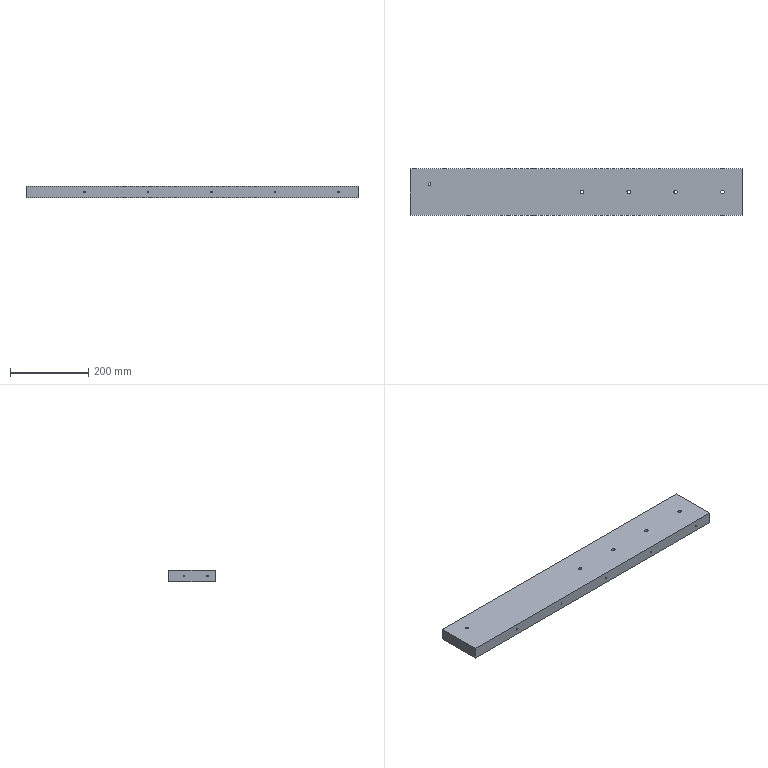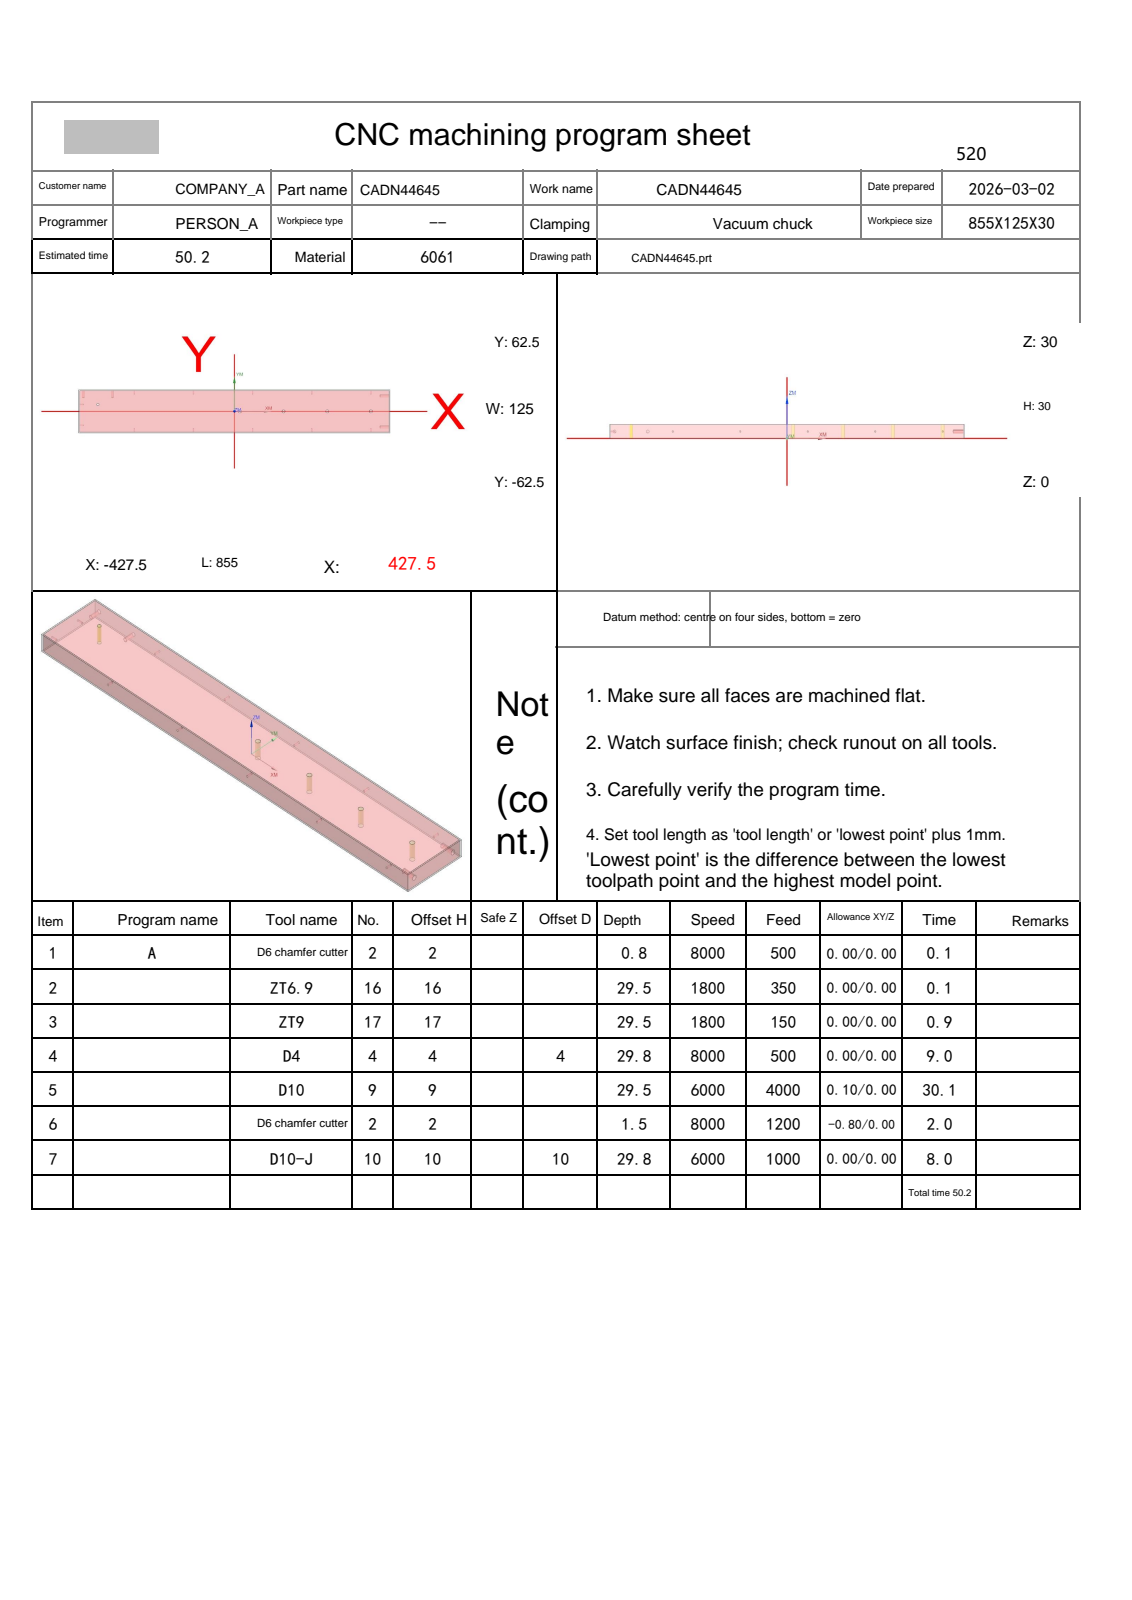NC program | NX | posted by the shop | part box 850 x 120 x 30 mm
Lines 1478 to 2164 of 2164:
N5 T09 M06
(D10  D=10. R=0. H=09 ce=0.10 di=0.00)
G00 G90 G54 X0.0 Y65.1 M03 S6000
G43 H09 Z80.
M08
Z30.5
G01 X425. Z30.392 F4000.
G02 X430.1 Y60. Z30.39 I0.0 J-5.1
G01 Y-60. Z30.36
G02 X425. Y-65.1 Z30.358 I-5.1 J0.0
G01 X-425. Z30.142
G02 X-430.1 Y-60. Z30.14 I0.0 J5.1
G01 Y60. Z30.11
G02 X-425. Y65.1 Z30.108 I5.1 J0.0
G01 X425. Z29.892
G02 X430.1 Y60. Z29.89 I0.0 J-5.1
G01 Y-60. Z29.86
G02 X425. Y-65.1 Z29.858 I-5.1 J0.0
G01 X-425. Z29.642
G02 X-430.1 Y-60. Z29.64 I0.0 J5.1
G01 Y60. Z29.61
G02 X-425. Y65.1 Z29.608 I5.1 J0.0
G01 X425. Z29.392
G02 X430.1 Y60. Z29.39 I0.0 J-5.1
G01 Y-60. Z29.36
G02 X425. Y-65.1 Z29.358 I-5.1 J0.0
G01 X-425. Z29.142
G02 X-430.1 Y-60. Z29.14 I0.0 J5.1
G01 Y60. Z29.11
G02 X-425. Y65.1 Z29.108 I5.1 J0.0
G01 X425. Z28.892
G02 X430.1 Y60. Z28.89 I0.0 J-5.1
G01 Y-60. Z28.86
G02 X425. Y-65.1 Z28.858 I-5.1 J0.0
G01 X-425. Z28.642
G02 X-430.1 Y-60. Z28.64 I0.0 J5.1
G01 Y60. Z28.61
G02 X-425. Y65.1 Z28.608 I5.1 J0.0
G01 X425. Z28.392
G02 X430.1 Y60. Z28.39 I0.0 J-5.1
G01 Y-60. Z28.36
G02 X425. Y-65.1 Z28.358 I-5.1 J0.0
G01 X-425. Z28.142
G02 X-430.1 Y-60. Z28.14 I0.0 J5.1
G01 Y60. Z28.11
G02 X-425. Y65.1 Z28.108 I5.1 J0.0
G01 X425. Z27.892
G02 X430.1 Y60. Z27.89 I0.0 J-5.1
G01 Y-60. Z27.86
G02 X425. Y-65.1 Z27.858 I-5.1 J0.0
G01 X-425. Z27.642
G02 X-430.1 Y-60. Z27.64 I0.0 J5.1
G01 Y60. Z27.61
G02 X-425. Y65.1 Z27.608 I5.1 J0.0
G01 X425. Z27.392
G02 X430.1 Y60. Z27.39 I0.0 J-5.1
G01 Y-60. Z27.36
G02 X425. Y-65.1 Z27.358 I-5.1 J0.0
G01 X-425. Z27.142
G02 X-430.1 Y-60. Z27.14 I0.0 J5.1
G01 Y60. Z27.11
G02 X-425. Y65.1 Z27.108 I5.1 J0.0
G01 X425. Z26.892
G02 X430.1 Y60. Z26.89 I0.0 J-5.1
G01 Y-60. Z26.86
G02 X425. Y-65.1 Z26.858 I-5.1 J0.0
G01 X-425. Z26.642
G02 X-430.1 Y-60. Z26.64 I0.0 J5.1
G01 Y60. Z26.61
G02 X-425. Y65.1 Z26.608 I5.1 J0.0
G01 X425. Z26.392
G02 X430.1 Y60. Z26.39 I0.0 J-5.1
G01 Y-60. Z26.36
G02 X425. Y-65.1 Z26.358 I-5.1 J0.0
G01 X-425. Z26.142
G02 X-430.1 Y-60. Z26.14 I0.0 J5.1
G01 Y60. Z26.11
G02 X-425. Y65.1 Z26.108 I5.1 J0.0
G01 X425. Z25.892
G02 X430.1 Y60. Z25.89 I0.0 J-5.1
G01 Y-60. Z25.86
G02 X425. Y-65.1 Z25.858 I-5.1 J0.0
G01 X-425. Z25.642
G02 X-430.1 Y-60. Z25.64 I0.0 J5.1
G01 Y60. Z25.61
G02 X-425. Y65.1 Z25.608 I5.1 J0.0
G01 X425. Z25.392
G02 X430.1 Y60. Z25.39 I0.0 J-5.1
G01 Y-60. Z25.36
G02 X425. Y-65.1 Z25.358 I-5.1 J0.0
G01 X-425. Z25.142
G02 X-430.1 Y-60. Z25.14 I0.0 J5.1
G01 Y60. Z25.11
G02 X-425. Y65.1 Z25.108 I5.1 J0.0
G01 X425. Z24.892
G02 X430.1 Y60. Z24.89 I0.0 J-5.1
G01 Y-60. Z24.86
G02 X425. Y-65.1 Z24.858 I-5.1 J0.0
G01 X-425. Z24.642
G02 X-430.1 Y-60. Z24.64 I0.0 J5.1
G01 Y60. Z24.61
G02 X-425. Y65.1 Z24.608 I5.1 J0.0
G01 X425. Z24.392
G02 X430.1 Y60. Z24.39 I0.0 J-5.1
G01 Y-60. Z24.36
G02 X425. Y-65.1 Z24.358 I-5.1 J0.0
G01 X-425. Z24.142
G02 X-430.1 Y-60. Z24.14 I0.0 J5.1
G01 Y60. Z24.11
G02 X-425. Y65.1 Z24.108 I5.1 J0.0
G01 X425. Z23.892
G02 X430.1 Y60. Z23.89 I0.0 J-5.1
G01 Y-60. Z23.86
G02 X425. Y-65.1 Z23.858 I-5.1 J0.0
G01 X-425. Z23.642
G02 X-430.1 Y-60. Z23.64 I0.0 J5.1
G01 Y60. Z23.61
G02 X-425. Y65.1 Z23.608 I5.1 J0.0
G01 X425. Z23.392
G02 X430.1 Y60. Z23.39 I0.0 J-5.1
G01 Y-60. Z23.36
G02 X425. Y-65.1 Z23.358 I-5.1 J0.0
G01 X-425. Z23.142
G02 X-430.1 Y-60. Z23.14 I0.0 J5.1
G01 Y60. Z23.11
G02 X-425. Y65.1 Z23.108 I5.1 J0.0
G01 X425. Z22.892
G02 X430.1 Y60. Z22.89 I0.0 J-5.1
G01 Y-60. Z22.86
G02 X425. Y-65.1 Z22.858 I-5.1 J0.0
G01 X-425. Z22.642
G02 X-430.1 Y-60. Z22.64 I0.0 J5.1
G01 Y60. Z22.61
G02 X-425. Y65.1 Z22.608 I5.1 J0.0
G01 X425. Z22.392
G02 X430.1 Y60. Z22.39 I0.0 J-5.1
G01 Y-60. Z22.36
G02 X425. Y-65.1 Z22.358 I-5.1 J0.0
G01 X-425. Z22.142
G02 X-430.1 Y-60. Z22.14 I0.0 J5.1
G01 Y60. Z22.11
G02 X-425. Y65.1 Z22.108 I5.1 J0.0
G01 X425. Z21.892
G02 X430.1 Y60. Z21.89 I0.0 J-5.1
G01 Y-60. Z21.86
G02 X425. Y-65.1 Z21.858 I-5.1 J0.0
G01 X-425. Z21.642
G02 X-430.1 Y-60. Z21.64 I0.0 J5.1
G01 Y60. Z21.61
G02 X-425. Y65.1 Z21.608 I5.1 J0.0
G01 X425. Z21.392
G02 X430.1 Y60. Z21.39 I0.0 J-5.1
G01 Y-60. Z21.36
G02 X425. Y-65.1 Z21.358 I-5.1 J0.0
G01 X-425. Z21.142
G02 X-430.1 Y-60. Z21.14 I0.0 J5.1
G01 Y60. Z21.11
G02 X-425. Y65.1 Z21.108 I5.1 J0.0
G01 X425. Z20.892
G02 X430.1 Y60. Z20.89 I0.0 J-5.1
G01 Y-60. Z20.86
G02 X425. Y-65.1 Z20.858 I-5.1 J0.0
G01 X-425. Z20.642
G02 X-430.1 Y-60. Z20.64 I0.0 J5.1
G01 Y60. Z20.61
G02 X-425. Y65.1 Z20.608 I5.1 J0.0
G01 X425. Z20.392
G02 X430.1 Y60. Z20.39 I0.0 J-5.1
G01 Y-60. Z20.36
G02 X425. Y-65.1 Z20.358 I-5.1 J0.0
G01 X-425. Z20.142
G02 X-430.1 Y-60. Z20.14 I0.0 J5.1
G01 Y60. Z20.11
G02 X-425. Y65.1 Z20.108 I5.1 J0.0
G01 X425. Z19.892
G02 X430.1 Y60. Z19.89 I0.0 J-5.1
G01 Y-60. Z19.86
G02 X425. Y-65.1 Z19.858 I-5.1 J0.0
G01 X-425. Z19.642
G02 X-430.1 Y-60. Z19.64 I0.0 J5.1
G01 Y60. Z19.61
G02 X-425. Y65.1 Z19.608 I5.1 J0.0
G01 X425. Z19.392
G02 X430.1 Y60. Z19.39 I0.0 J-5.1
G01 Y-60. Z19.36
G02 X425. Y-65.1 Z19.358 I-5.1 J0.0
G01 X-425. Z19.142
G02 X-430.1 Y-60. Z19.14 I0.0 J5.1
G01 Y60. Z19.11
G02 X-425. Y65.1 Z19.108 I5.1 J0.0
G01 X425. Z18.892
G02 X430.1 Y60. Z18.89 I0.0 J-5.1
G01 Y-60. Z18.86
G02 X425. Y-65.1 Z18.858 I-5.1 J0.0
G01 X-425. Z18.642
G02 X-430.1 Y-60. Z18.64 I0.0 J5.1
G01 Y60. Z18.61
G02 X-425. Y65.1 Z18.608 I5.1 J0.0
G01 X425. Z18.392
G02 X430.1 Y60. Z18.39 I0.0 J-5.1
G01 Y-60. Z18.36
G02 X425. Y-65.1 Z18.358 I-5.1 J0.0
G01 X-425. Z18.142
G02 X-430.1 Y-60. Z18.14 I0.0 J5.1
G01 Y60. Z18.11
G02 X-425. Y65.1 Z18.108 I5.1 J0.0
G01 X425. Z17.892
G02 X430.1 Y60. Z17.89 I0.0 J-5.1
G01 Y-60. Z17.86
G02 X425. Y-65.1 Z17.858 I-5.1 J0.0
G01 X-425. Z17.642
G02 X-430.1 Y-60. Z17.64 I0.0 J5.1
G01 Y60. Z17.61
G02 X-425. Y65.1 Z17.608 I5.1 J0.0
G01 X425. Z17.392
G02 X430.1 Y60. Z17.39 I0.0 J-5.1
G01 Y-60. Z17.36
G02 X425. Y-65.1 Z17.358 I-5.1 J0.0
G01 X-425. Z17.142
G02 X-430.1 Y-60. Z17.14 I0.0 J5.1
G01 Y60. Z17.11
G02 X-425. Y65.1 Z17.108 I5.1 J0.0
G01 X425. Z16.892
G02 X430.1 Y60. Z16.89 I0.0 J-5.1
G01 Y-60. Z16.86
G02 X425. Y-65.1 Z16.858 I-5.1 J0.0
G01 X-425. Z16.642
G02 X-430.1 Y-60. Z16.64 I0.0 J5.1
G01 Y60. Z16.61
G02 X-425. Y65.1 Z16.608 I5.1 J0.0
G01 X425. Z16.392
G02 X430.1 Y60. Z16.39 I0.0 J-5.1
G01 Y-60. Z16.36
G02 X425. Y-65.1 Z16.358 I-5.1 J0.0
G01 X-425. Z16.142
G02 X-430.1 Y-60. Z16.14 I0.0 J5.1
G01 Y60. Z16.11
G02 X-425. Y65.1 Z16.108 I5.1 J0.0
G01 X425. Z15.892
G02 X430.1 Y60. Z15.89 I0.0 J-5.1
G01 Y-60. Z15.86
G02 X425. Y-65.1 Z15.858 I-5.1 J0.0
G01 X-425. Z15.642
G02 X-430.1 Y-60. Z15.64 I0.0 J5.1
G01 Y60. Z15.61
G02 X-425. Y65.1 Z15.608 I5.1 J0.0
G01 X425. Z15.392
G02 X430.1 Y60. Z15.39 I0.0 J-5.1
G01 Y-60. Z15.36
G02 X425. Y-65.1 Z15.358 I-5.1 J0.0
G01 X-425. Z15.142
G02 X-430.1 Y-60. Z15.14 I0.0 J5.1
G01 Y60. Z15.11
G02 X-425. Y65.1 Z15.108 I5.1 J0.0
G01 X425. Z14.892
G02 X430.1 Y60. Z14.89 I0.0 J-5.1
G01 Y-60. Z14.86
G02 X425. Y-65.1 Z14.858 I-5.1 J0.0
G01 X-425. Z14.642
G02 X-430.1 Y-60. Z14.64 I0.0 J5.1
G01 Y60. Z14.61
G02 X-425. Y65.1 Z14.608 I5.1 J0.0
G01 X425. Z14.392
G02 X430.1 Y60. Z14.39 I0.0 J-5.1
G01 Y-60. Z14.36
G02 X425. Y-65.1 Z14.358 I-5.1 J0.0
G01 X-425. Z14.142
G02 X-430.1 Y-60. Z14.14 I0.0 J5.1
G01 Y60. Z14.11
G02 X-425. Y65.1 Z14.108 I5.1 J0.0
G01 X425. Z13.892
G02 X430.1 Y60. Z13.89 I0.0 J-5.1
G01 Y-60. Z13.86
G02 X425. Y-65.1 Z13.858 I-5.1 J0.0
G01 X-425. Z13.642
G02 X-430.1 Y-60. Z13.64 I0.0 J5.1
G01 Y60. Z13.61
G02 X-425. Y65.1 Z13.608 I5.1 J0.0
G01 X425. Z13.392
G02 X430.1 Y60. Z13.39 I0.0 J-5.1
G01 Y-60. Z13.36
G02 X425. Y-65.1 Z13.358 I-5.1 J0.0
G01 X-425. Z13.142
G02 X-430.1 Y-60. Z13.14 I0.0 J5.1
G01 Y60. Z13.11
G02 X-425. Y65.1 Z13.108 I5.1 J0.0
G01 X425. Z12.892
G02 X430.1 Y60. Z12.89 I0.0 J-5.1
G01 Y-60. Z12.86
G02 X425. Y-65.1 Z12.858 I-5.1 J0.0
G01 X-425. Z12.642
G02 X-430.1 Y-60. Z12.64 I0.0 J5.1
G01 Y60. Z12.61
G02 X-425. Y65.1 Z12.608 I5.1 J0.0
G01 X425. Z12.392
G02 X430.1 Y60. Z12.39 I0.0 J-5.1
G01 Y-60. Z12.36
G02 X425. Y-65.1 Z12.358 I-5.1 J0.0
G01 X-425. Z12.142
G02 X-430.1 Y-60. Z12.14 I0.0 J5.1
G01 Y60. Z12.11
G02 X-425. Y65.1 Z12.108 I5.1 J0.0
G01 X425. Z11.892
G02 X430.1 Y60. Z11.89 I0.0 J-5.1
G01 Y-60. Z11.86
G02 X425. Y-65.1 Z11.858 I-5.1 J0.0
G01 X-425. Z11.642
G02 X-430.1 Y-60. Z11.64 I0.0 J5.1
G01 Y60. Z11.61
G02 X-425. Y65.1 Z11.608 I5.1 J0.0
G01 X425. Z11.392
G02 X430.1 Y60. Z11.39 I0.0 J-5.1
G01 Y-60. Z11.36
G02 X425. Y-65.1 Z11.358 I-5.1 J0.0
G01 X-425. Z11.142
G02 X-430.1 Y-60. Z11.14 I0.0 J5.1
G01 Y60. Z11.11
G02 X-425. Y65.1 Z11.108 I5.1 J0.0
G01 X425. Z10.892
G02 X430.1 Y60. Z10.89 I0.0 J-5.1
G01 Y-60. Z10.86
G02 X425. Y-65.1 Z10.858 I-5.1 J0.0
G01 X-425. Z10.642
G02 X-430.1 Y-60. Z10.64 I0.0 J5.1
G01 Y60. Z10.61
G02 X-425. Y65.1 Z10.608 I5.1 J0.0
G01 X425. Z10.392
G02 X430.1 Y60. Z10.39 I0.0 J-5.1
G01 Y-60. Z10.36
G02 X425. Y-65.1 Z10.358 I-5.1 J0.0
G01 X-425. Z10.142
G02 X-430.1 Y-60. Z10.14 I0.0 J5.1
G01 Y60. Z10.11
G02 X-425. Y65.1 Z10.108 I5.1 J0.0
G01 X425. Z9.892
G02 X430.1 Y60. Z9.89 I0.0 J-5.1
G01 Y-60. Z9.86
G02 X425. Y-65.1 Z9.858 I-5.1 J0.0
G01 X-425. Z9.642
G02 X-430.1 Y-60. Z9.64 I0.0 J5.1
G01 Y60. Z9.61
G02 X-425. Y65.1 Z9.608 I5.1 J0.0
G01 X425. Z9.392
G02 X430.1 Y60. Z9.39 I0.0 J-5.1
G01 Y-60. Z9.36
G02 X425. Y-65.1 Z9.358 I-5.1 J0.0
G01 X-425. Z9.142
G02 X-430.1 Y-60. Z9.14 I0.0 J5.1
G01 Y60. Z9.11
G02 X-425. Y65.1 Z9.108 I5.1 J0.0
G01 X425. Z8.892
G02 X430.1 Y60. Z8.89 I0.0 J-5.1
G01 Y-60. Z8.86
G02 X425. Y-65.1 Z8.858 I-5.1 J0.0
G01 X-425. Z8.642
G02 X-430.1 Y-60. Z8.64 I0.0 J5.1
G01 Y60. Z8.61
G02 X-425. Y65.1 Z8.608 I5.1 J0.0
G01 X425. Z8.392
G02 X430.1 Y60. Z8.39 I0.0 J-5.1
G01 Y-60. Z8.36
G02 X425. Y-65.1 Z8.358 I-5.1 J0.0
G01 X-425. Z8.142
G02 X-430.1 Y-60. Z8.14 I0.0 J5.1
G01 Y60. Z8.11
G02 X-425. Y65.1 Z8.108 I5.1 J0.0
G01 X425. Z7.892
G02 X430.1 Y60. Z7.89 I0.0 J-5.1
G01 Y-60. Z7.86
G02 X425. Y-65.1 Z7.858 I-5.1 J0.0
G01 X-425. Z7.642
G02 X-430.1 Y-60. Z7.64 I0.0 J5.1
G01 Y60. Z7.61
G02 X-425. Y65.1 Z7.608 I5.1 J0.0
G01 X425. Z7.392
G02 X430.1 Y60. Z7.39 I0.0 J-5.1
G01 Y-60. Z7.36
G02 X425. Y-65.1 Z7.358 I-5.1 J0.0
G01 X-425. Z7.142
G02 X-430.1 Y-60. Z7.14 I0.0 J5.1
G01 Y60. Z7.11
G02 X-425. Y65.1 Z7.108 I5.1 J0.0
G01 X425. Z6.892
G02 X430.1 Y60. Z6.89 I0.0 J-5.1
G01 Y-60. Z6.86
G02 X425. Y-65.1 Z6.858 I-5.1 J0.0
G01 X-425. Z6.642
G02 X-430.1 Y-60. Z6.64 I0.0 J5.1
G01 Y60. Z6.61
G02 X-425. Y65.1 Z6.608 I5.1 J0.0
G01 X425. Z6.392
G02 X430.1 Y60. Z6.39 I0.0 J-5.1
G01 Y-60. Z6.36
G02 X425. Y-65.1 Z6.358 I-5.1 J0.0
G01 X-425. Z6.142
G02 X-430.1 Y-60. Z6.14 I0.0 J5.1
G01 Y60. Z6.11
G02 X-425. Y65.1 Z6.108 I5.1 J0.0
G01 X425. Z5.892
G02 X430.1 Y60. Z5.89 I0.0 J-5.1
G01 Y-60. Z5.86
G02 X425. Y-65.1 Z5.858 I-5.1 J0.0
G01 X-425. Z5.642
G02 X-430.1 Y-60. Z5.64 I0.0 J5.1
G01 Y60. Z5.61
G02 X-425. Y65.1 Z5.608 I5.1 J0.0
G01 X425. Z5.392
G02 X430.1 Y60. Z5.39 I0.0 J-5.1
G01 Y-60. Z5.36
G02 X425. Y-65.1 Z5.358 I-5.1 J0.0
G01 X-425. Z5.142
G02 X-430.1 Y-60. Z5.14 I0.0 J5.1
G01 Y60. Z5.11
G02 X-425. Y65.1 Z5.108 I5.1 J0.0
G01 X425. Z4.892
G02 X430.1 Y60. Z4.89 I0.0 J-5.1
G01 Y-60. Z4.86
G02 X425. Y-65.1 Z4.858 I-5.1 J0.0
G01 X-425. Z4.642
G02 X-430.1 Y-60. Z4.64 I0.0 J5.1
G01 Y60. Z4.61
G02 X-425. Y65.1 Z4.608 I5.1 J0.0
G01 X425. Z4.392
G02 X430.1 Y60. Z4.39 I0.0 J-5.1
G01 Y-60. Z4.36
G02 X425. Y-65.1 Z4.358 I-5.1 J0.0
G01 X-425. Z4.142
G02 X-430.1 Y-60. Z4.14 I0.0 J5.1
G01 Y60. Z4.11
G02 X-425. Y65.1 Z4.108 I5.1 J0.0
G01 X425. Z3.892
G02 X430.1 Y60. Z3.89 I0.0 J-5.1
G01 Y-60. Z3.86
G02 X425. Y-65.1 Z3.858 I-5.1 J0.0
G01 X-425. Z3.642
G02 X-430.1 Y-60. Z3.64 I0.0 J5.1
G01 Y60. Z3.61
G02 X-425. Y65.1 Z3.608 I5.1 J0.0
G01 X425. Z3.392
G02 X430.1 Y60. Z3.39 I0.0 J-5.1
G01 Y-60. Z3.36
G02 X425. Y-65.1 Z3.358 I-5.1 J0.0
G01 X-425. Z3.142
G02 X-430.1 Y-60. Z3.14 I0.0 J5.1
G01 Y60. Z3.11
G02 X-425. Y65.1 Z3.108 I5.1 J0.0
G01 X425. Z2.892
G02 X430.1 Y60. Z2.89 I0.0 J-5.1
G01 Y-60. Z2.86
G02 X425. Y-65.1 Z2.858 I-5.1 J0.0
G01 X-425. Z2.642
G02 X-430.1 Y-60. Z2.64 I0.0 J5.1
G01 Y60. Z2.61
G02 X-425. Y65.1 Z2.608 I5.1 J0.0
G01 X425. Z2.392
G02 X430.1 Y60. Z2.39 I0.0 J-5.1
G01 Y-60. Z2.36
G02 X425. Y-65.1 Z2.358 I-5.1 J0.0
G01 X-425. Z2.142
G02 X-430.1 Y-60. Z2.14 I0.0 J5.1
G01 Y60. Z2.11
G02 X-425. Y65.1 Z2.108 I5.1 J0.0
G01 X425. Z1.892
G02 X430.1 Y60. Z1.89 I0.0 J-5.1
G01 Y-60. Z1.86
G02 X425. Y-65.1 Z1.858 I-5.1 J0.0
G01 X-425. Z1.642
G02 X-430.1 Y-60. Z1.64 I0.0 J5.1
G01 Y60. Z1.61
G02 X-425. Y65.1 Z1.608 I5.1 J0.0
G01 X425. Z1.392
G02 X430.1 Y60. Z1.39 I0.0 J-5.1
G01 Y-60. Z1.36
G02 X425. Y-65.1 Z1.358 I-5.1 J0.0
G01 X-425. Z1.142
G02 X-430.1 Y-60. Z1.14 I0.0 J5.1
G01 Y60. Z1.11
G02 X-425. Y65.1 Z1.108 I5.1 J0.0
G01 X425. Z.892
G02 X430.1 Y60. Z.89 I0.0 J-5.1
G01 Y-60. Z.86
G02 X425. Y-65.1 Z.858 I-5.1 J0.0
G01 X-425. Z.642
G02 X-430.1 Y-60. Z.64 I0.0 J5.1
G01 Y60. Z.61
G02 X-425. Y65.1 Z.608 I5.1 J0.0
G01 X0.0 Z.5
X425.
G02 X430.1 Y60. I0.0 J-5.1
G01 Y-60.
G02 X425. Y-65.1 I-5.1 J0.0
G01 X-425.
G02 X-430.1 Y-60. I0.0 J5.1
G01 Y60.
G02 X-425. Y65.1 I5.1 J0.0
G01 X0.0
X.5
Z1.5
G00 Z80.
G91 G28 Z0.0
M05
M09
G91 G28 Z0.0
M01
N6 T02 M06
(D6 chamfer cutter  D=6. R=0. H=02 ce=0.00 di=0.00)
G00 G90 G54 X.25 Y-62.128 M03 S6000
G43 H02 Z80.
M08
Z32.099
G01 Z28.5 F1200.
G03 X.33 Y-61.828 I-.52 J.3
X.03 Y-61.308 I-.6 J0.0
G01 X0.0 Y-61.3
X-425.
G02 X-426.3 Y-60. I0.0 J1.3
G01 Y59.999
G02 X-425. Y61.3 I1.3 J0.0
G01 X425.
G02 X426.3 Y60. I0.0 J-1.3
G01 Y-60.
G02 X425. Y-61.3 I-1.3 J0.0
G01 X0.0
X-.03 Y-61.308
G03 X-.33 Y-61.828 I.3 J-.52
X-.25 Y-62.128 I.6 J0.0
G01 Z32.099
G00 Z80.
G00 G90 X-373.834 Y18.5 M03 S8000
Z80.
Z29.2
G01 Z28.7 F500.
X-373.6
G03 X-372.1 Y20. I0.0 J1.5
X-375. Y22.9 I-2.9 J0.0
X-377.9 Y20. I0.0 J-2.9
X-375. Y17.1 I2.9 J0.0
X-372.1 Y20. I0.0 J2.9
X-373.6 Y21.5 I-1.5 J0.0
G01 X-373.834
Z29.2
G00 Z80.
G00 G90 X14.279 Y2.705 M03 S8000
Z80.
Z29.5
G01 Z29. F600.
X14.2 Y3.
G03 X11.2 Y0.0 I0.0 J-3.
X15. Y-3.8 I3.8 J0.0
X18.8 Y0.0 I0.0 J3.8
X15. Y3.8 I-3.8 J0.0
X11.2 Y0.0 I0.0 J-3.8
X14.2 Y-3. I3. J0.0
G01 X14.279 Y-2.705
Z29.5
G00 Z80.
X134.279 Y2.705
Z29.5
G01 Z29.
X134.2 Y3.
G03 X131.2 Y0.0 I0.0 J-3.
X135. Y-3.8 I3.8 J0.0
X138.8 Y0.0 I0.0 J3.8
X135. Y3.8 I-3.8 J0.0
X131.2 Y0.0 I0.0 J-3.8
X134.2 Y-3. I3. J0.0
G01 X134.279 Y-2.705
Z29.5
G00 Z80.
X254.279 Y2.705
Z29.5
G01 Z29.
X254.2 Y3.
G03 X251.2 Y0.0 I0.0 J-3.
X255. Y-3.8 I3.8 J0.0
X258.8 Y0.0 I0.0 J3.8
X255. Y3.8 I-3.8 J0.0
X251.2 Y0.0 I0.0 J-3.8
X254.2 Y-3. I3. J0.0
G01 X254.279 Y-2.705
Z29.5
G00 Z80.
X374.279 Y2.705
Z29.5
G01 Z29.
X374.2 Y3.
G03 X371.2 Y0.0 I0.0 J-3.
X375. Y-3.8 I3.8 J0.0
X378.8 Y0.0 I0.0 J3.8
X375. Y3.8 I-3.8 J0.0
X371.2 Y0.0 I0.0 J-3.8
X374.2 Y-3. I3. J0.0
G01 X374.279 Y-2.705
Z29.5
G00 Z80.
G91 G28 Z0.0
M05
M09
G91 G28 Z0.0
M01
N7 T10 M06
(D10-J  D=10. R=0. H=10 ce=0.00 di=0.00)
G00 G90 G54 X-426.013 Y66.116 M03 S6000
G43 H10 Z80.
M08
Z20.667
G01 Z20.167 F1000.
G41 D10
X-425.997 Y65.917
G03 X-425. Y65. I.997 J.083
G01 X425.
G02 X430. Y60. I0.0 J-5.
G01 Y-60.
G02 X425. Y-65. I-5. J0.0
G01 X-425.
G02 X-430. Y-60. I0.0 J5.
G01 Y60.
G02 X-425. Y65. I5. J0.0
G01 X-424.5
G03 X-423.5 Y66. I0.0 J1.
G01 G40 Y66.2
Z20.667
G00 Z80.
X-426.013 Y66.116
Z10.833
G01 Z10.333
G41 D10
X-425.997 Y65.917
G03 X-425. Y65. I.997 J.083
G01 X425.
G02 X430. Y60. I0.0 J-5.
G01 Y-60.
G02 X425. Y-65. I-5. J0.0
G01 X-425.
G02 X-430. Y-60. I0.0 J5.
G01 Y60.
G02 X-425. Y65. I5. J0.0
G01 X-424.5
G03 X-423.5 Y66. I0.0 J1.
G01 G40 Y66.2
Z10.833
G00 Z80.
X-426.013 Y66.116
Z1.
G01 Z.5
G41 D10
X-425.997 Y65.917
G03 X-425. Y65. I.997 J.083
G01 X425.
G02 X430. Y60. I0.0 J-5.
G01 Y-60.
G02 X425. Y-65. I-5. J0.0
G01 X-425.
G02 X-430. Y-60. I0.0 J5.
G01 Y60.
G02 X-425. Y65. I5. J0.0
G01 X-424.5
G03 X-423.5 Y66. I0.0 J1.
G01 G40 Y66.2
Z1.
G00 Z80.
G00 G90 X-426.005 Y66.016 M03 S6000
Z80.
Z.7
G01 Z.2 F1000.
G41 D10
X-425.997 Y65.917
G03 X-425. Y65. I.997 J.083
G01 X425.
G02 X430. Y60. I0.0 J-5.
G01 Y-60.
G02 X425. Y-65. I-5. J0.0
G01 X-425.
G02 X-430. Y-60. I0.0 J5.
G01 Y60.
G02 X-425. Y65. I5. J0.0
G01 X-424.5
G03 X-423.5 Y66. I0.0 J1.
G01 G40 Y66.1
Z.7
G00 Z80.
M05
M09
G91 G28 Z0.0
G91 G28 Y0.0
M30
%